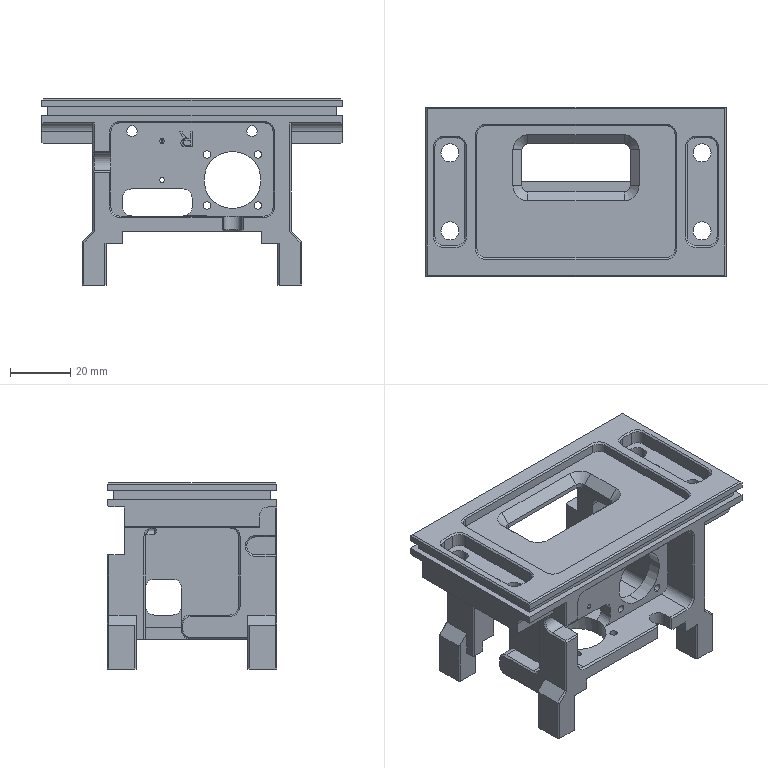NC program | Mastercam | posted with a generic post | part box 100 x 56.5 x 62 mm
Lines 31428 to 33708 of 47040, first 1881 of 2281 lines:
N7300 T16 M6
N7310 G0 G90 G17 G54 X59.62 Y2.263 A0. S5000 M3
N7320 G43 H16 Z20. M8
N7330 Z1.
N7340 G1 Z-28.5 F600.
N7350 X58.489 Y1.131 F1000.
N7360 G3 X58.02 Y0. I1.131 J-1.131
N7370 G1 Y-31.
N7380 G2 X50. Y-39.02 I-8.02 J0.
N7390 G1 X-50.
N7400 G2 X-58.02 Y-31. I0. J8.02
N7410 G1 Y31.
N7420 G2 X-50. Y39.02 I8.02 J0.
N7430 G1 X50.
N7440 G2 X58.02 Y31. I0. J-8.02
N7450 G1 Y0.
N7460 Y-.5
N7470 G3 X58.489 Y-1.631 I1.6 J0.
N7480 G1 X59.62 Y-2.763
N7490 G0 Z20.
N7500 Y2.263
N7510 Z1.
N7520 G1 Z-28.5 F600.
N7530 X58.489 Y1.131 F1000.
N7540 G3 X58.02 Y0. I1.131 J-1.131
N7550 G1 Y-31.
N7560 G2 X50. Y-39.02 I-8.02 J0.
N7570 G1 X-50.
N7580 G2 X-58.02 Y-31. I0. J8.02
N7590 G1 Y31.
N7600 G2 X-50. Y39.02 I8.02 J0.
N7610 G1 X50.
N7620 G2 X58.02 Y31. I0. J-8.02
N7630 G1 Y0.
N7640 Y-.5
N7650 G3 X58.489 Y-1.631 I1.6 J0.
N7660 G1 X59.62 Y-2.763
N7670 Y2.263
N7680 Z-57. F600.
N7690 X58.489 Y1.131 F1000.
N7700 G3 X58.02 Y0. I1.131 J-1.131
N7710 G1 Y-31.
N7720 G2 X50. Y-39.02 I-8.02 J0.
N7730 G1 X-50.
N7740 G2 X-58.02 Y-31. I0. J8.02
N7750 G1 Y31.
N7760 G2 X-50. Y39.02 I8.02 J0.
N7770 G1 X50.
N7780 G2 X58.02 Y31. I0. J-8.02
N7790 G1 Y0.
N7800 Y-.5
N7810 G3 X58.489 Y-1.631 I1.6 J0.
N7820 G1 X59.62 Y-2.763
N7830 G0 Z20.
N7840 Y2.263
N7850 Z-27.5
N7860 G1 Z-57. F600.
N7870 X58.489 Y1.131 F1000.
N7880 G3 X58.02 Y0. I1.131 J-1.131
N7890 G1 Y-31.
N7900 G2 X50. Y-39.02 I-8.02 J0.
N7910 G1 X-50.
N7920 G2 X-58.02 Y-31. I0. J8.02
N7930 G1 Y31.
N7940 G2 X-50. Y39.02 I8.02 J0.
N7950 G1 X50.
N7960 G2 X58.02 Y31. I0. J-8.02
N7970 G1 Y0.
N7980 Y-.5
N7990 G3 X58.489 Y-1.631 I1.6 J0.
N8000 G1 X59.62 Y-2.763
N8010 G0 Z20.
N8020 M5
N8030 G91 G28 Z0. M9
N8040 A0.
N8050 M01
N8060 T5 M6
N8070 G0 G90 G17 G54 X50. Y-31.65 A0. S6500 M3
N8080 G43 H5 Z20. M8
N8090 Z1.
N8100 G1 Z-.75 F600.
N8110 X-50. F1000.
N8120 G2 X-50.65 Y-31. I0. J.65
N8130 G1 Y31.
N8140 G2 X-50. Y31.65 I.65 J0.
N8150 G1 X50.
N8160 G2 X50.65 Y31. I0. J-.65
N8170 G1 Y-31.
N8180 G2 X50. Y-31.65 I-.65 J0.
N8190 G0 Z20.
N8200 Y-26.15
N8210 Z1.
N8220 G1 Z-.75 F600.
N8230 X-50. F1000.
N8240 G0 Z20.
N8250 Y-27.85
N8260 Z1.
N8270 G1 Z-.75 F600.
N8280 X50. F1000.
N8290 G0 Z20.
N8300 X-13.5 Y4.85
N8310 Z1.
N8320 G1 Z-12.75 F600.
N8330 G3 X-22.35 Y-4. I0. J-8.85 F1000.
N8340 X-13.5 Y-12.85 I8.85 J0.
N8350 X-4.65 Y-4. I0. J8.85
N8360 X-13.5 Y4.85 I-8.85 J0.
N8370 G0 Z20.
N8380 X.65 Y5.
N8390 Z1.
N8400 G1 Z-12.75 F600.
N8410 Y2. F1000.
N8420 G3 X3. Y-.35 I2.35 J0.
N8430 G1 X20.2
N8440 G3 X22.55 Y2. I0. J2.35
N8450 G1 Y5.
N8460 G0 Z20.
N8470 X12.166 Y6.95
N8480 Z1.
N8490 G1 Z-1. F600.
N8500 X11.883 Y7.232 F1000.
N8510 G3 X11.6 Y7.35 I-.283 J-.282
N8520 G1 X2.926
N8530 X-24.
N8540 G3 X-26.35 Y5. I0. J-2.35
N8550 G1 Y-20.
N8560 G3 X-24. Y-22.35 I2.35 J0.
N8570 G1 X24.
N8580 G3 X26.35 Y-20. I0. J2.35
N8590 G1 Y5.
N8600 G3 X24. Y7.35 I-2.35 J0.
N8610 G1 X20.274
N8620 X11.6
N8630 X11.1
N8640 G3 X10.817 Y7.232 I0. J-.4
N8650 G1 X10.534 Y6.95
N8660 G0 Z20.
N8670 S6000 M3
N8680 X-22. Y4.5
N8690 G98 G81 Z-12.7 R-11. F200.
N8700 Y-12.5
N8710 X-5. Y4.5
N8720 Y-12.5
N8730 X10. Y-4.
N8740 Y-17.
N8750 X-20. Y-20.3
N8760 X20.
N8770 G80
N8780 M5
N8790 G91 G0 G28 Z0. M9
N8800 A0.
N8810 M01
N8820 T20 M6
N8830 G0 G90 G17 G54 X-104.75 Y23.248 A0. S4000 M3
N8840 G43 H20 Z20. M8
N8850 Z11.
N8860 G1 Z9.34 F600.
N8870 X73.25 F2000.
N8880 G2 X96.498 Y0. I0. J-23.248
N8890 X73.25 Y-23.248 I-23.248 J0.
N8900 G1 X-104.75
N8910 G0 Z20.
N8920 Y23.248
N8930 Z10.34
N8940 G1 Z8.68 F600.
N8950 X73.25 F2000.
N8960 G2 X96.498 Y0. I0. J-23.248
N8970 X73.25 Y-23.248 I-23.248 J0.
N8980 G1 X-104.75
N8990 G0 Z20.
N9000 Y23.248
N9010 Z9.68
N9020 G1 Z8.02 F600.
N9030 X73.25 F2000.
N9040 G2 X96.498 Y0. I0. J-23.248
N9050 X73.25 Y-23.248 I-23.248 J0.
N9060 G1 X-104.75
N9070 G0 Z20.
N9080 Y23.248
N9090 Z9.02
N9100 G1 Z7.36 F600.
N9110 X73.25 F2000.
N9120 G2 X96.498 Y0. I0. J-23.248
N9130 X73.25 Y-23.248 I-23.248 J0.
N9140 G1 X-104.75
N9150 G0 Z20.
N9160 Y23.248
N9170 Z8.36
N9180 G1 Z6.7 F600.
N9190 X73.25 F2000.
N9200 G2 X96.498 Y0. I0. J-23.248
N9210 X73.25 Y-23.248 I-23.248 J0.
N9220 G1 X-104.75
N9230 G0 Z20.
N9240 Y23.248
N9250 Z7.7
N9260 G1 Z6.04 F600.
N9270 X73.25 F2000.
N9280 G2 X96.498 Y0. I0. J-23.248
N9290 X73.25 Y-23.248 I-23.248 J0.
N9300 G1 X-104.75
N9310 G0 Z20.
N9320 Y23.248
N9330 Z7.04
N9340 G1 Z5.38 F600.
N9350 X73.25 F2000.
N9360 G2 X96.498 Y0. I0. J-23.248
N9370 X73.25 Y-23.248 I-23.248 J0.
N9380 G1 X-104.75
N9390 G0 Z20.
N9400 Y23.248
N9410 Z6.38
N9420 G1 Z4.72 F600.
N9430 X73.25 F2000.
N9440 G2 X96.498 Y0. I0. J-23.248
N9450 X73.25 Y-23.248 I-23.248 J0.
N9460 G1 X-104.75
N9470 G0 Z20.
N9480 Y23.248
N9490 Z5.72
N9500 G1 Z4.06 F600.
N9510 X73.25 F2000.
N9520 G2 X96.498 Y0. I0. J-23.248
N9530 X73.25 Y-23.248 I-23.248 J0.
N9540 G1 X-104.75
N9550 G0 Z20.
N9560 Y23.248
N9570 Z5.06
N9580 G1 Z3.4 F600.
N9590 X73.25 F2000.
N9600 G2 X96.498 Y0. I0. J-23.248
N9610 X73.25 Y-23.248 I-23.248 J0.
N9620 G1 X-104.75
N9630 G0 Z20.
N9640 Y23.248
N9650 Z4.4
N9660 G1 Z2.74 F600.
N9670 X73.25 F2000.
N9680 G2 X96.498 Y0. I0. J-23.248
N9690 X73.25 Y-23.248 I-23.248 J0.
N9700 G1 X-104.75
N9710 G0 Z20.
N9720 Y23.248
N9730 Z3.74
N9740 G1 Z2.08 F600.
N9750 X73.25 F2000.
N9760 G2 X96.498 Y0. I0. J-23.248
N9770 X73.25 Y-23.248 I-23.248 J0.
N9780 G1 X-104.75
N9790 G0 Z20.
N9800 Y23.248
N9810 Z3.08
N9820 G1 Z1.42 F600.
N9830 X73.25 F2000.
N9840 G2 X96.498 Y0. I0. J-23.248
N9850 X73.25 Y-23.248 I-23.248 J0.
N9860 G1 X-104.75
N9870 G0 Z20.
N9880 Y23.248
N9890 Z2.42
N9900 G1 Z.76 F600.
N9910 X73.25 F2000.
N9920 G2 X96.498 Y0. I0. J-23.248
N9930 X73.25 Y-23.248 I-23.248 J0.
N9940 G1 X-104.75
N9950 G0 Z20.
N9960 Y23.248
N9970 Z1.76
N9980 G1 Z.1 F600.
N9990 X73.25 F2000.
N100 G2 X96.498 Y0. I0. J-23.248
N110 X73.25 Y-23.248 I-23.248 J0.
N120 G1 X-104.75
N130 G0 Z20.
N140 Y23.248
N150 Z1.1
N160 G1 Z0. F600.
N170 X73.25 F1000.
N180 G2 X96.498 Y0. I0. J-23.248
N190 X73.25 Y-23.248 I-23.248 J0.
N200 G1 X-104.75
N210 G0 Z20.
N220 M5
N230 G91 G28 Z0. M9
N240 A0.
N250 M01
N260 T11 M6
N270 G0 G90 G17 G54 X57. Y-13.1 A0. S8000 M3
N280 G43 H11 Z20. M8
N290 Z1.
N300 G1 Z-.628 F600.
N310 X50. F4000.
N320 X-50.
N330 X-57.
N340 Z-1.256 F600.
N350 X-50. F4000.
N360 X50.
N370 X57.
N380 Z-1.883 F600.
N390 X50. F4000.
N400 X-50.
N410 X-57.
N420 Z-2.511 F600.
N430 X-50. F4000.
N440 X50.
N450 X57.
N460 Z-3.139 F600.
N470 X50. F4000.
N480 X-50.
N490 X-57.
N500 Z-3.767 F600.
N510 X-50. F4000.
N520 X50.
N530 X57.
N540 Z-4.394 F600.
N550 X50. F4000.
N560 X-50.
N570 X-57.
N580 Z-5.022 F600.
N590 X-50. F4000.
N600 X50.
N610 X57.
N620 Z-5.65 F600.
N630 X50. F4000.
N640 X-50.
N650 X-57.
N660 G0 Z20.
N670 Y-16.9
N680 Z1.
N690 G1 Z-.628 F600.
N700 X-50. F4000.
N710 X50.
N720 X57.
N730 Z-1.256 F600.
N740 X50. F4000.
N750 X-50.
N760 X-57.
N770 Z-1.883 F600.
N780 X-50. F4000.
N790 X50.
N800 X57.
N810 Z-2.511 F600.
N820 X50. F4000.
N830 X-50.
N840 X-57.
N850 Z-3.139 F600.
N860 X-50. F4000.
N870 X50.
N880 X57.
N890 Z-3.767 F600.
N900 X50. F4000.
N910 X-50.
N920 X-57.
N930 Z-4.394 F600.
N940 X-50. F4000.
N950 X50.
N960 X57.
N970 Z-5.022 F600.
N980 X50. F4000.
N990 X-50.
N1000 X-57.
N1010 Z-5.65 F600.
N1020 X-50. F4000.
N1030 X50.
N1040 X57.
N1050 G0 Z20.
N1060 M5
N1070 G91 G28 Z0. M9
N1080 A0.
N1090 M01
N1100 T12 M6
N1110 G0 G90 G17 G54 X57. Y-13. A0. S8000 M3
N1120 G43 H12 Z20. M8
N1130 Z-4.75
N1140 G1 Z-5.75 F600.
N1150 X50. F1000.
N1160 X-50.
N1170 X-57.
N1180 G0 Z20.
N1190 Y-17.
N1200 Z-4.75
N1210 G1 Z-5.75 F600.
N1220 X-50. F1000.
N1230 X50.
N1240 X57.
N1250 G0 Z20.
N1260 M5
N1270 G91 G28 Z0. M9
N1280 A0.
N1290 M01
N1300 T11 M6
N1310 G0 G90 G17 G54 X2.228 Y-2.835 A0. S8000 M3
N1320 G43 H11 Z20. M8
N1330 Z1.
N1340 G1 Z.325 F600.
N1350 G3 X7.628 Y2.565 Z.073 I0. J5.4 F4000.
N1360 X2.228 Y7.965 Z-.18 I-5.4 J0.
N1370 X-3.172 Y2.565 Z-.432 I0. J-5.4
N1380 X2.228 Y-2.835 Z-.685 I5.4 J0.
N1390 G1 X3.035
N1400 Y-1.165
N1410 X0.
N1420 X-3.035
N1430 Y-2.835
N1440 X2.228
N1450 G2 X2.953 Y-3.418 I0. J-.743
N1460 G1 X3.73 Y-6.941
N1470 G3 X4.455 Y-7.523 I.725 J.16
N1480 G1 X7.723
N1490 Y3.523
N1500 X0.
N1510 X-7.723
N1520 Y-7.523
N1530 X4.455
N1540 G2 X5.18 Y-8.106 I0. J-.743
N1550 G1 X5.957 Y-11.629
N1560 G3 X6.683 Y-12.212 I.726 J.16
N1570 G1 X12.412
N1580 Y8.212
N1590 X0.
N1600 X-12.412
N1610 Y-12.212
N1620 X6.683
N1630 G2 X7.408 Y-12.794 I0. J-.742
N1640 G1 X8.185 Y-16.317
N1650 G3 X8.91 Y-16.9 I.725 J.16
N1660 G1 X17.099
N1670 X17.1 Y12.656
N1680 X17.087 Y12.887
N1690 X16.959 Y12.898
N1700 X0. Y12.9
N1710 X-16.188
N1720 X-17.087 Y12.887
N1730 X-17.1 Y12.656
N1740 Y-16.898
N1750 X-17.099 Y-16.9
N1760 X8.91
N1770 G0 Z20.
N1780 X2.228 Y-2.835
N1790 Z.315
N1800 G1 Z-.36 F600.
N1810 G3 X7.628 Y2.565 Z-.612 I0. J5.4 F4000.
N1820 X2.228 Y7.965 Z-.865 I-5.4 J0.
N1830 X-3.172 Y2.565 Z-1.117 I0. J-5.4
N1840 X2.228 Y-2.835 Z-1.369 I5.4 J0.
N1850 G1 X3.035
N1860 Y-1.165
N1870 X0.
N1880 X-3.035
N1890 Y-2.835
N1900 X2.228
N1910 G2 X2.953 Y-3.418 I0. J-.743
N1920 G1 X3.73 Y-6.941
N1930 G3 X4.455 Y-7.523 I.725 J.16
N1940 G1 X7.723
N1950 Y3.523
N1960 X0.
N1970 X-7.723
N1980 Y-7.523
N1990 X4.455
N2000 G2 X5.18 Y-8.106 I0. J-.743
N2010 G1 X5.957 Y-11.629
N2020 G3 X6.683 Y-12.212 I.726 J.16
N2030 G1 X12.412
N2040 Y8.212
N2050 X0.
N2060 X-12.412
N2070 Y-12.212
N2080 X6.683
N2090 G2 X7.408 Y-12.794 I0. J-.742
N2100 G1 X8.185 Y-16.317
N2110 G3 X8.91 Y-16.9 I.725 J.16
N2120 G1 X17.099
N2130 X17.1 Y12.656
N2140 X17.087 Y12.887
N2150 X16.959 Y12.898
N2160 X0. Y12.9
N2170 X-16.188
N2180 X-17.087 Y12.887
N2190 X-17.1 Y12.656
N2200 Y-16.898
N2210 X-17.099 Y-16.9
N2220 X8.91
N2230 G0 Z20.
N2240 X2.228 Y-2.835
N2250 Z-.369
N2260 G1 Z-1.044 F600.
N2270 G3 X7.628 Y2.565 Z-1.297 I0. J5.4 F4000.
N2280 X2.228 Y7.965 Z-1.549 I-5.4 J0.
N2290 X-3.172 Y2.565 Z-1.802 I0. J-5.4
N2300 X2.228 Y-2.835 Z-2.054 I5.4 J0.
N2310 G1 X3.035
N2320 Y-1.165
N2330 X0.
N2340 X-3.035
N2350 Y-2.835
N2360 X2.228
N2370 G2 X2.953 Y-3.418 I0. J-.743
N2380 G1 X3.73 Y-6.941
N2390 G3 X4.455 Y-7.523 I.725 J.16
N2400 G1 X7.723
N2410 Y3.523
N2420 X0.
N2430 X-7.723
N2440 Y-7.523
N2450 X4.455
N2460 G2 X5.18 Y-8.106 I0. J-.743
N2470 G1 X5.957 Y-11.629
N2480 G3 X6.683 Y-12.212 I.726 J.16
N2490 G1 X12.412
N2500 Y8.212
N2510 X0.
N2520 X-12.412
N2530 Y-12.212
N2540 X6.683
N2550 G2 X7.408 Y-12.794 I0. J-.742
N2560 G1 X8.185 Y-16.317
N2570 G3 X8.91 Y-16.9 I.725 J.16
N2580 G1 X17.099
N2590 X17.1 Y12.656
N2600 X17.087 Y12.887
N2610 X16.959 Y12.898
N2620 X0. Y12.9
N2630 X-16.188
N2640 X-17.087 Y12.887
N2650 X-17.1 Y12.656
N2660 Y-16.898
N2670 X-17.099 Y-16.9
N2680 X8.91
N2690 G0 Z20.
N2700 X2.228 Y-2.835
N2710 Z-1.054
N2720 G1 Z-1.729 F600.
N2730 G3 X7.628 Y2.565 Z-1.982 I0. J5.4 F4000.
N2740 X2.228 Y7.965 Z-2.234 I-5.4 J0.
N2750 X-3.172 Y2.565 Z-2.486 I0. J-5.4
N2760 X2.228 Y-2.835 Z-2.739 I5.4 J0.
N2770 G1 X3.035
N2780 Y-1.165
N2790 X0.
N2800 X-3.035
N2810 Y-2.835
N2820 X2.228
N2830 G2 X2.953 Y-3.418 I0. J-.743
N2840 G1 X3.73 Y-6.941
N2850 G3 X4.455 Y-7.523 I.725 J.16
N2860 G1 X7.723
N2870 Y3.523
N2880 X0.
N2890 X-7.723
N2900 Y-7.523
N2910 X4.455
N2920 G2 X5.18 Y-8.106 I0. J-.743
N2930 G1 X5.957 Y-11.629
N2940 G3 X6.683 Y-12.212 I.726 J.16
N2950 G1 X12.412
N2960 Y8.212
N2970 X0.
N2980 X-12.412
N2990 Y-12.212
N3000 X6.683
N3010 G2 X7.408 Y-12.794 I0. J-.742
N3020 G1 X8.185 Y-16.317
N3030 G3 X8.91 Y-16.9 I.725 J.16
N3040 G1 X17.099
N3050 X17.1 Y12.656
N3060 X17.087 Y12.887
N3070 X16.959 Y12.898
N3080 X0. Y12.9
N3090 X-16.188
N3100 X-17.087 Y12.887
N3110 X-17.1 Y12.656
N3120 Y-16.898
N3130 X-17.099 Y-16.9
N3140 X8.91
N3150 G0 Z20.
N3160 X2.228 Y-2.835
N3170 Z-1.739
N3180 G1 Z-2.414 F600.
N3190 G3 X7.628 Y2.565 Z-2.666 I0. J5.4 F4000.
N3200 X2.228 Y7.965 Z-2.919 I-5.4 J0.
N3210 X-3.172 Y2.565 Z-3.171 I0. J-5.4
N3220 X2.228 Y-2.835 Z-3.424 I5.4 J0.
N3230 G1 X3.035
N3240 Y-1.165
N3250 X0.
N3260 X-3.035
N3270 Y-2.835
N3280 X2.228
N3290 G2 X2.953 Y-3.418 I0. J-.743
N3300 G1 X3.73 Y-6.941
N3310 G3 X4.455 Y-7.523 I.725 J.16
N3320 G1 X7.723
N3330 Y3.523
N3340 X0.
N3350 X-7.723
N3360 Y-7.523
N3370 X4.455
N3380 G2 X5.18 Y-8.106 I0. J-.743
N3390 G1 X5.957 Y-11.629
N3400 G3 X6.683 Y-12.212 I.726 J.16
N3410 G1 X12.412
N3420 Y8.212
N3430 X0.
N3440 X-12.412
N3450 Y-12.212
N3460 X6.683
N3470 G2 X7.408 Y-12.794 I0. J-.742
N3480 G1 X8.185 Y-16.317
N3490 G3 X8.91 Y-16.9 I.725 J.16
N3500 G1 X17.099
N3510 X17.1 Y12.656
N3520 X17.087 Y12.887
N3530 X16.959 Y12.898
N3540 X0. Y12.9
N3550 X-16.188
N3560 X-17.087 Y12.887
N3570 X-17.1 Y12.656
N3580 Y-16.898
N3590 X-17.099 Y-16.9
N3600 X8.91
N3610 G0 Z20.
N3620 X2.228 Y-2.835
N3630 Z-2.424
N3640 G1 Z-3.099 F600.
N3650 G3 X7.628 Y2.565 Z-3.351 I0. J5.4 F4000.
N3660 X2.228 Y7.965 Z-3.603 I-5.4 J0.
N3670 X-3.172 Y2.565 Z-3.856 I0. J-5.4
N3680 X2.228 Y-2.835 Z-4.108 I5.4 J0.
N3690 G1 X3.035
N3700 Y-1.165
N3710 X0.
N3720 X-3.035
N3730 Y-2.835
N3740 X2.228
N3750 G2 X2.953 Y-3.418 I0. J-.743
N3760 G1 X3.73 Y-6.941
N3770 G3 X4.455 Y-7.523 I.725 J.16
N3780 G1 X7.723
N3790 Y3.523
N3800 X0.
N3810 X-7.723
N3820 Y-7.523
N3830 X4.455
N3840 G2 X5.18 Y-8.106 I0. J-.743
N3850 G1 X5.957 Y-11.629
N3860 G3 X6.683 Y-12.212 I.726 J.16
N3870 G1 X12.412
N3880 Y8.212
N3890 X0.
N3900 X-12.412
N3910 Y-12.212
N3920 X6.683
N3930 G2 X7.408 Y-12.794 I0. J-.742
N3940 G1 X8.185 Y-16.317
N3950 G3 X8.91 Y-16.9 I.725 J.16
N3960 G1 X17.099
N3970 X17.1 Y12.656
N3980 X17.087 Y12.887
N3990 X16.959 Y12.898
N4000 X0. Y12.9
N4010 X-16.188
N4020 X-17.087 Y12.887
N4030 X-17.1 Y12.656
N4040 Y-16.898
N4050 X-17.099 Y-16.9
N4060 X8.91
N4070 G0 Z20.
N4080 X2.228 Y-2.835
N4090 Z-3.108
N4100 G1 Z-3.783 F600.
N4110 G3 X7.628 Y2.565 Z-4.036 I0. J5.4 F4000.
N4120 X2.228 Y7.965 Z-4.288 I-5.4 J0.
N4130 X-3.172 Y2.565 Z-4.541 I0. J-5.4
N4140 X2.228 Y-2.835 Z-4.793 I5.4 J0.
N4150 G1 X3.035
N4160 Y-1.165
N4170 X0.
N4180 X-3.035
N4190 Y-2.835
N4200 X2.228
N4210 G2 X2.953 Y-3.418 I0. J-.743
N4220 G1 X3.73 Y-6.941
N4230 G3 X4.455 Y-7.523 I.725 J.16
N4240 G1 X7.723
N4250 Y3.523
N4260 X0.
N4270 X-7.723
N4280 Y-7.523
N4290 X4.455
N4300 G2 X5.18 Y-8.106 I0. J-.743
N4310 G1 X5.957 Y-11.629
N4320 G3 X6.683 Y-12.212 I.726 J.16
N4330 G1 X12.412
N4340 Y8.212
N4350 X0.
N4360 X-12.412
N4370 Y-12.212
N4380 X6.683
N4390 G2 X7.408 Y-12.794 I0. J-.742
N4400 G1 X8.185 Y-16.317
N4410 G3 X8.91 Y-16.9 I.725 J.16
N4420 G1 X17.099
N4430 X17.1 Y12.656
N4440 X17.087 Y12.887
N4450 X16.959 Y12.898
N4460 X0. Y12.9
N4470 X-16.188
N4480 X-17.087 Y12.887
N4490 X-17.1 Y12.656
N4500 Y-16.898
N4510 X-17.099 Y-16.9
N4520 X8.91
N4530 G0 Z20.
N4540 X2.228 Y-2.835
N4550 Z-3.793
N4560 G1 Z-4.468 F600.
N4570 G3 X7.628 Y2.565 Z-4.72 I0. J5.4 F4000.
N4580 X2.228 Y7.965 Z-4.973 I-5.4 J0.
N4590 X-3.172 Y2.565 Z-5.225 I0. J-5.4
N4600 X2.228 Y-2.835 Z-5.478 I5.4 J0.
N4610 G1 X3.035
N4620 Y-1.165
N4630 X0.
N4640 X-3.035
N4650 Y-2.835
N4660 X2.228
N4670 G2 X2.953 Y-3.418 I0. J-.743
N4680 G1 X3.73 Y-6.941
N4690 G3 X4.455 Y-7.523 I.725 J.16
N4700 G1 X7.723
N4710 Y3.523
N4720 X0.
N4730 X-7.723
N4740 Y-7.523
N4750 X4.455
N4760 G2 X5.18 Y-8.106 I0. J-.743
N4770 G1 X5.957 Y-11.629
N4780 G3 X6.683 Y-12.212 I.726 J.16
N4790 G1 X12.412
N4800 Y8.212
N4810 X0.
N4820 X-12.412
N4830 Y-12.212
N4840 X6.683
N4850 G2 X7.408 Y-12.794 I0. J-.742
N4860 G1 X8.185 Y-16.317
N4870 G3 X8.91 Y-16.9 I.725 J.16
N4880 G1 X17.099
N4890 X17.1 Y12.656
N4900 X17.087 Y12.887
N4910 X16.959 Y12.898
N4920 X0. Y12.9
N4930 X-16.188
N4940 X-17.087 Y12.887
N4950 X-17.1 Y12.656
N4960 Y-16.898
N4970 X-17.099 Y-16.9
N4980 X8.91
N4990 G0 Z20.
N5000 X2.228 Y-2.835
N5010 Z-4.478
N5020 G1 Z-5.153 F600.
N5030 G3 X7.628 Y2.565 Z-5.405 I0. J5.4 F4000.
N5040 X2.228 Y7.965 Z-5.658 I-5.4 J0.
N5050 X-3.172 Y2.565 Z-5.91 I0. J-5.4
N5060 X2.228 Y-2.835 Z-6.162 I5.4 J0.
N5070 G1 X3.035
N5080 Y-1.165
N5090 X0.
N5100 X-3.035
N5110 Y-2.835
N5120 X2.228
N5130 G2 X2.953 Y-3.418 I0. J-.743
N5140 G1 X3.73 Y-6.941
N5150 G3 X4.455 Y-7.523 I.725 J.16
N5160 G1 X7.723
N5170 Y3.523
N5180 X0.
N5190 X-7.723
N5200 Y-7.523
N5210 X4.455
N5220 G2 X5.18 Y-8.106 I0. J-.743
N5230 G1 X5.957 Y-11.629
N5240 G3 X6.683 Y-12.212 I.726 J.16
N5250 G1 X12.412
N5260 Y8.212
N5270 X0.
N5280 X-12.412
N5290 Y-12.212
N5300 X6.683
N5310 G2 X7.408 Y-12.794 I0. J-.742
N5320 G1 X8.185 Y-16.317
N5330 G3 X8.91 Y-16.9 I.725 J.16
N5340 G1 X17.099
N5350 X17.1 Y12.656
N5360 X17.087 Y12.887
N5370 X16.959 Y12.898
N5380 X0. Y12.9
N5390 X-16.188
N5400 X-17.087 Y12.887
N5410 X-17.1 Y12.656
N5420 Y-16.898
N5430 X-17.099 Y-16.9
N5440 X8.91
N5450 G0 Z20.
N5460 X2.228 Y-2.835
N5470 Z-5.162
N5480 G1 Z-5.838 F600.
N5490 G3 X7.628 Y2.565 Z-6.09 I0. J5.4 F4000.
N5500 X2.228 Y7.965 Z-6.342 I-5.4 J0.
N5510 X-3.172 Y2.565 Z-6.595 I0. J-5.4
N5520 X2.228 Y-2.835 Z-6.847 I5.4 J0.
N5530 G1 X3.035
N5540 Y-1.165
N5550 X0.
N5560 X-3.035
N5570 Y-2.835
N5580 X2.228
N5590 G2 X2.953 Y-3.418 I0. J-.743
N5600 G1 X3.73 Y-6.941
N5610 G3 X4.455 Y-7.523 I.725 J.16
N5620 G1 X7.723
N5630 Y3.523
N5640 X0.
N5650 X-7.723
N5660 Y-7.523
N5670 X4.455
N5680 G2 X5.18 Y-8.106 I0. J-.743
N5690 G1 X5.957 Y-11.629
N5700 G3 X6.683 Y-12.212 I.726 J.16
N5710 G1 X12.412
N5720 Y8.212
N5730 X0.
N5740 X-12.412
N5750 Y-12.212
N5760 X6.683
N5770 G2 X7.408 Y-12.794 I0. J-.742
N5780 G1 X8.185 Y-16.317
N5790 G3 X8.91 Y-16.9 I.725 J.16
N5800 G1 X17.099
N5810 X17.1 Y12.656
N5820 X17.087 Y12.887
N5830 X16.959 Y12.898
N5840 X0. Y12.9
N5850 X-16.188
N5860 X-17.087 Y12.887
N5870 X-17.1 Y12.656
N5880 Y-16.898
N5890 X-17.099 Y-16.9
N5900 X8.91
N5910 G0 Z20.
N5920 X2.228 Y-2.835
N5930 Z-5.847
N5940 G1 Z-6.522 F600.
N5950 G3 X7.628 Y2.565 Z-6.775 I0. J5.4 F4000.
N5960 X2.228 Y7.965 Z-7.027 I-5.4 J0.
N5970 X-3.172 Y2.565 Z-7.28 I0. J-5.4
N5980 X2.228 Y-2.835 Z-7.532 I5.4 J0.
N5990 G1 X3.035
N6000 Y-1.165
N6010 X0.
N6020 X-3.035
N6030 Y-2.835
N6040 X2.228
N6050 G2 X2.953 Y-3.418 I0. J-.743
N6060 G1 X3.73 Y-6.941
N6070 G3 X4.455 Y-7.523 I.725 J.16
N6080 G1 X7.723
N6090 Y3.523
N6100 X0.
N6110 X-7.723
N6120 Y-7.523
N6130 X4.455
N6140 G2 X5.18 Y-8.106 I0. J-.743
N6150 G1 X5.957 Y-11.629
N6160 G3 X6.683 Y-12.212 I.726 J.16
N6170 G1 X12.412
N6180 Y8.212
N6190 X0.
N6200 X-12.412
N6210 Y-12.212
N6220 X6.683
N6230 G2 X7.408 Y-12.794 I0. J-.742
N6240 G1 X8.185 Y-16.317
N6250 G3 X8.91 Y-16.9 I.725 J.16
N6260 G1 X17.099
N6270 X17.1 Y12.656
N6280 X17.087 Y12.887
N6290 X16.959 Y12.898
N6300 X0. Y12.9
N6310 X-16.188
N6320 X-17.087 Y12.887
N6330 X-17.1 Y12.656
N6340 Y-16.898
N6350 X-17.099 Y-16.9
N6360 X8.91
N6370 G0 Z20.
N6380 X2.228 Y-2.835
N6390 Z-6.532
N6400 G1 Z-7.207 F600.
N6410 G3 X7.628 Y2.565 Z-7.459 I0. J5.4 F4000.
N6420 X2.228 Y7.965 Z-7.712 I-5.4 J0.
N6430 X-3.172 Y2.565 Z-7.964 I0. J-5.4
N6440 X2.228 Y-2.835 Z-8.217 I5.4 J0.
N6450 G1 X3.035
N6460 Y-1.165
N6470 X0.
N6480 X-3.035
N6490 Y-2.835
N6500 X2.228
N6510 G2 X2.953 Y-3.418 I0. J-.743
N6520 G1 X3.73 Y-6.941
N6530 G3 X4.455 Y-7.523 I.725 J.16
N6540 G1 X7.723
N6550 Y3.523
N6560 X0.
N6570 X-7.723
N6580 Y-7.523
N6590 X4.455
N6600 G2 X5.18 Y-8.106 I0. J-.743
N6610 G1 X5.957 Y-11.629
N6620 G3 X6.683 Y-12.212 I.726 J.16
N6630 G1 X12.412
N6640 Y8.212
N6650 X0.
N6660 X-12.412
N6670 Y-12.212
N6680 X6.683
N6690 G2 X7.408 Y-12.794 I0. J-.742
N6700 G1 X8.185 Y-16.317
N6710 G3 X8.91 Y-16.9 I.725 J.16
N6720 G1 X17.099
N6730 X17.1 Y12.656
N6740 X17.087 Y12.887
N6750 X16.959 Y12.898
N6760 X0. Y12.9
N6770 X-16.188
N6780 X-17.087 Y12.887
N6790 X-17.1 Y12.656
N6800 Y-16.898
N6810 X-17.099 Y-16.9
N6820 X8.91
N6830 G0 Z20.
N6840 X2.228 Y-2.835
N6850 Z-7.217
N6860 G1 Z-7.892 F600.
N6870 G3 X7.628 Y2.565 Z-8.144 I0. J5.4 F4000.
N6880 X2.228 Y7.965 Z-8.397 I-5.4 J0.
N6890 X-3.172 Y2.565 Z-8.649 I0. J-5.4
N6900 X2.228 Y-2.835 Z-8.901 I5.4 J0.
N6910 G1 X3.035
N6920 Y-1.165
N6930 X0.
N6940 X-3.035
N6950 Y-2.835
N6960 X2.228
N6970 G2 X2.953 Y-3.418 I0. J-.743
N6980 G1 X3.73 Y-6.941
N6990 G3 X4.455 Y-7.523 I.725 J.16
N7000 G1 X7.723
N7010 Y3.523
N7020 X0.
N7030 X-7.723
N7040 Y-7.523
N7050 X4.455
N7060 G2 X5.18 Y-8.106 I0. J-.743
N7070 G1 X5.957 Y-11.629
N7080 G3 X6.683 Y-12.212 I.726 J.16
N7090 G1 X12.412
N7100 Y8.212
N7110 X0.
N7120 X-12.412
N7130 Y-12.212
N7140 X6.683
N7150 G2 X7.408 Y-12.794 I0. J-.742
N7160 G1 X8.185 Y-16.317
N7170 G3 X8.91 Y-16.9 I.725 J.16
N7180 G1 X17.099
N7190 X17.1 Y12.656
N7200 X17.087 Y12.887
N7210 X16.959 Y12.898
N7220 X0. Y12.9
N7230 X-16.188
N7240 X-17.087 Y12.887
N7250 X-17.1 Y12.656
N7260 Y-16.898
N7270 X-17.099 Y-16.9
N7280 X8.91
N7290 G0 Z20.
N7300 X2.228 Y-2.835
N7310 Z-7.901
N7320 G1 Z-8.576 F600.
N7330 G3 X7.628 Y2.565 Z-8.829 I0. J5.4 F4000.
N7340 X2.228 Y7.965 Z-9.081 I-5.4 J0.
N7350 X-3.172 Y2.565 Z-9.334 I0. J-5.4
N7360 X2.228 Y-2.835 Z-9.586 I5.4 J0.
N7370 G1 X3.035
N7380 Y-1.165
N7390 X0.
N7400 X-3.035
N7410 Y-2.835
N7420 X2.228
N7430 G2 X2.953 Y-3.418 I0. J-.743
N7440 G1 X3.73 Y-6.941
N7450 G3 X4.455 Y-7.523 I.725 J.16
N7460 G1 X7.723
N7470 Y3.523
N7480 X0.
N7490 X-7.723
N7500 Y-7.523
N7510 X4.455
N7520 G2 X5.18 Y-8.106 I0. J-.743
N7530 G1 X5.957 Y-11.629
N7540 G3 X6.683 Y-12.212 I.726 J.16
N7550 G1 X12.412
N7560 Y8.212
N7570 X0.
N7580 X-12.412
N7590 Y-12.212
N7600 X6.683
N7610 G2 X7.408 Y-12.794 I0. J-.742
N7620 G1 X8.185 Y-16.317
N7630 G3 X8.91 Y-16.9 I.725 J.16
N7640 G1 X17.099
N7650 X17.1 Y12.656
N7660 X17.087 Y12.887
N7670 X16.959 Y12.898
N7680 X0. Y12.9
N7690 X-16.188
N7700 X-17.087 Y12.887
N7710 X-17.1 Y12.656
N7720 Y-16.898
N7730 X-17.099 Y-16.9
N7740 X8.91
N7750 G0 Z20.
N7760 X2.228 Y-2.835
N7770 Z-8.586
N7780 G1 Z-9.261 F600.
N7790 G3 X7.628 Y2.565 Z-9.514 I0. J5.4 F4000.
N7800 X2.228 Y7.965 Z-9.766 I-5.4 J0.
N7810 X-3.172 Y2.565 Z-10.018 I0. J-5.4
N7820 X2.228 Y-2.835 Z-10.271 I5.4 J0.
N7830 G1 X3.035
N7840 Y-1.165
N7850 X0.
N7860 X-3.035
N7870 Y-2.835
N7880 X2.228
N7890 G2 X2.953 Y-3.418 I0. J-.743
N7900 G1 X3.73 Y-6.941
N7910 G3 X4.455 Y-7.523 I.725 J.16
N7920 G1 X7.723
N7930 Y3.523
N7940 X0.
N7950 X-7.723
N7960 Y-7.523
N7970 X4.455
N7980 G2 X5.18 Y-8.106 I0. J-.743
N7990 G1 X5.957 Y-11.629
N8000 G3 X6.683 Y-12.212 I.726 J.16
N8010 G1 X12.412
N8020 Y8.212
N8030 X0.
N8040 X-12.412
N8050 Y-12.212
N8060 X6.683
N8070 G2 X7.408 Y-12.794 I0. J-.742
N8080 G1 X8.185 Y-16.317
N8090 G3 X8.91 Y-16.9 I.725 J.16
N8100 G1 X17.099
N8110 X17.1 Y12.656
N8120 X17.087 Y12.887
N8130 X16.959 Y12.898
N8140 X0. Y12.9
N8150 X-16.188
N8160 X-17.087 Y12.887
N8170 X-17.1 Y12.656
N8180 Y-16.898
N8190 X-17.099 Y-16.9
N8200 X8.91
N8210 G0 Z20.
N8220 X2.228 Y-2.835
N8230 Z-9.271
N8240 G1 Z-9.946 F600.
N8250 G3 X7.628 Y2.565 Z-10.198 I0. J5.4 F4000.
N8260 X2.228 Y7.965 Z-10.451 I-5.4 J0.
N8270 X-3.172 Y2.565 Z-10.703 I0. J-5.4
N8280 X2.228 Y-2.835 Z-10.956 I5.4 J0.
N8290 G1 X3.035
N8300 Y-1.165
N8310 X0.
N8320 X-3.035
N8330 Y-2.835
N8340 X2.228
N8350 G2 X2.953 Y-3.418 I0. J-.743
N8360 G1 X3.73 Y-6.941
N8370 G3 X4.455 Y-7.523 I.725 J.16
N8380 G1 X7.723
N8390 Y3.523
N8400 X0.
N8410 X-7.723
N8420 Y-7.523
N8430 X4.455
N8440 G2 X5.18 Y-8.106 I0. J-.743
N8450 G1 X5.957 Y-11.629
N8460 G3 X6.683 Y-12.212 I.726 J.16
N8470 G1 X12.412
N8480 Y8.212
N8490 X0.
N8500 X-12.412
N8510 Y-12.212
N8520 X6.683
N8530 G2 X7.408 Y-12.794 I0. J-.742
N8540 G1 X8.185 Y-16.317
N8550 G3 X8.91 Y-16.9 I.725 J.16
N8560 G1 X17.099
N8570 X17.1 Y12.656
N8580 X17.087 Y12.887
N8590 X16.959 Y12.898
N8600 X0. Y12.9
N8610 X-16.188
N8620 X-17.087 Y12.887
N8630 X-17.1 Y12.656
N8640 Y-16.898
N8650 X-17.099 Y-16.9
N8660 X8.91
N8670 G0 Z20.
N8680 X2.228 Y-2.835
N8690 Z-9.956
N8700 G1 Z-10.631 F600.
N8710 G3 X7.628 Y2.565 Z-10.883 I0. J5.4 F4000.
N8720 X2.228 Y7.965 Z-11.135 I-5.4 J0.
N8730 X-3.172 Y2.565 Z-11.388 I0. J-5.4
N8740 X2.228 Y-2.835 Z-11.64 I5.4 J0.
N8750 G1 X3.035
N8760 Y-1.165
N8770 X0.
N8780 X-3.035
N8790 Y-2.835
N8800 X2.228
N8810 G2 X2.953 Y-3.418 I0. J-.743
N8820 G1 X3.73 Y-6.941
N8830 G3 X4.455 Y-7.523 I.725 J.16
N8840 G1 X7.723
N8850 Y3.523
N8860 X0.
N8870 X-7.723
N8880 Y-7.523
N8890 X4.455
N8900 G2 X5.18 Y-8.106 I0. J-.743
N8910 G1 X5.957 Y-11.629
N8920 G3 X6.683 Y-12.212 I.726 J.16
N8930 G1 X12.412
N8940 Y8.212
N8950 X0.
N8960 X-12.412
N8970 Y-12.212
N8980 X6.683
N8990 G2 X7.408 Y-12.794 I0. J-.742
N9000 G1 X8.185 Y-16.317
N9010 G3 X8.91 Y-16.9 I.725 J.16
N9020 G1 X17.099
N9030 X17.1 Y12.656
N9040 X17.087 Y12.887
N9050 X16.959 Y12.898
N9060 X0. Y12.9
N9070 X-16.188
N9080 X-17.087 Y12.887
N9090 X-17.1 Y12.656
N9100 Y-16.898
N9110 X-17.099 Y-16.9
N9120 X8.91
N9130 G0 Z20.
N9140 X2.228 Y-2.835
N9150 Z-10.64
N9160 G1 Z-11.315 F600.
N9170 G3 X7.628 Y2.565 Z-11.568 I0. J5.4 F4000.
N9180 X2.228 Y7.965 Z-11.82 I-5.4 J0.
N9190 X-3.172 Y2.565 Z-12.073 I0. J-5.4
N9200 X2.228 Y-2.835 Z-12.325 I5.4 J0.
N9210 G1 X3.035
N9220 Y-1.165
N9230 X0.
N9240 X-3.035
N9250 Y-2.835
N9260 X2.228
N9270 G2 X2.953 Y-3.418 I0. J-.743
N9280 G1 X3.73 Y-6.941
N9290 G3 X4.455 Y-7.523 I.725 J.16
N9300 G1 X7.723
N9310 Y3.523
N9320 X0.
N9330 X-7.723
N9340 Y-7.523
N9350 X4.455
N9360 G2 X5.18 Y-8.106 I0. J-.743
N9370 G1 X5.957 Y-11.629
N9380 G3 X6.683 Y-12.212 I.726 J.16
N9390 G1 X12.412
N9400 Y8.212
N9410 X0.
N9420 X-12.412
N9430 Y-12.212
N9440 X6.683
N9450 G2 X7.408 Y-12.794 I0. J-.742
N9460 G1 X8.185 Y-16.317
N9470 G3 X8.91 Y-16.9 I.725 J.16
N9480 G1 X17.099
N9490 X17.1 Y12.656
N9500 X17.087 Y12.887
N9510 X16.959 Y12.898
N9520 X0. Y12.9
N9530 X-16.188
N9540 X-17.087 Y12.887
N9550 X-17.1 Y12.656
N9560 Y-16.898
N9570 X-17.099 Y-16.9
N9580 X8.91
N9590 G0 Z20.
N9600 X2.228 Y-2.835
N9610 Z-11.325
N9620 G1 Z-12. F600.
N9630 G3 X7.628 Y2.565 Z-12.252 I0. J5.4 F4000.
N9640 X2.228 Y7.965 Z-12.505 I-5.4 J0.
N9650 X-3.172 Y2.565 Z-12.757 I0. J-5.4
N9660 X2.228 Y-2.835 Z-13.01 I5.4 J0.
N9670 G1 X3.035
N9680 Y-1.165
N9690 X0.
N9700 X-3.035
N9710 Y-2.835
N9720 X2.228
N9730 G2 X2.953 Y-3.418 I0. J-.743
N9740 G1 X3.73 Y-6.941
N9750 G3 X4.455 Y-7.523 I.725 J.16
N9760 G1 X7.723
N9770 Y3.523
N9780 X0.
N9790 X-7.723
N9800 Y-7.523
N9810 X4.455
N9820 G2 X5.18 Y-8.106 I0. J-.743
N9830 G1 X5.957 Y-11.629
N9840 G3 X6.683 Y-12.212 I.726 J.16
N9850 G1 X12.412
N9860 Y8.212
N9870 X0.
N9880 X-12.412
N9890 Y-12.212
N9900 X6.683
N9910 G2 X7.408 Y-12.794 I0. J-.742
N9920 G1 X8.185 Y-16.317
N9930 G3 X8.91 Y-16.9 I.725 J.16
N9940 G1 X17.099
N9950 X17.1 Y12.656
N9960 X17.087 Y12.887
N9970 X16.959 Y12.898
N9980 X0. Y12.9
N9990 X-16.188
N100 X-17.087 Y12.887
N110 X-17.1 Y12.656
N120 Y-16.898
N130 X-17.099 Y-16.9
N140 X8.91
N150 G0 Z20.
N160 X2.228 Y-2.835
N170 Z-12.01
N180 G1 Z-12.685 F600.
N190 G3 X7.628 Y2.565 Z-12.937 I0. J5.4 F4000.
N200 X2.228 Y7.965 Z-13.19 I-5.4 J0.
N210 X-3.172 Y2.565 Z-13.442 I0. J-5.4
N220 X2.228 Y-2.835 Z-13.694 I5.4 J0.
N230 G1 X3.035
N240 Y-1.165
N250 X0.
N260 X-3.035
N270 Y-2.835
N280 X2.228
N290 G2 X2.953 Y-3.418 I0. J-.743
N300 G1 X3.73 Y-6.941
N310 G3 X4.455 Y-7.523 I.725 J.16
N320 G1 X7.723
N330 Y3.523
N340 X0.
N350 X-7.723
N360 Y-7.523
N370 X4.455
N380 G2 X5.18 Y-8.106 I0. J-.743
N390 G1 X5.957 Y-11.629
N400 G3 X6.683 Y-12.212 I.726 J.16
N410 G1 X12.412
N420 Y8.212
N430 X0.
N440 X-12.412
N450 Y-12.212
N460 X6.683
N470 G2 X7.408 Y-12.794 I0. J-.742
N480 G1 X8.185 Y-16.317
N490 G3 X8.91 Y-16.9 I.725 J.16
N500 G1 X17.099
N510 X17.1 Y12.656
N520 X17.087 Y12.887
N530 X16.959 Y12.898
N540 X0. Y12.9
N550 X-16.188
N560 X-17.087 Y12.887
N570 X-17.1 Y12.656
N580 Y-16.898
N590 X-17.099 Y-16.9
N600 X8.91
N610 G0 Z20.
N620 X2.228 Y-2.835
N630 Z-12.694
N640 G1 Z-13.369 F600.
N650 G3 X7.628 Y2.565 Z-13.622 I0. J5.4 F4000.
N660 X2.228 Y7.965 Z-13.874 I-5.4 J0.
N670 X-3.172 Y2.565 Z-14.127 I0. J-5.4
N680 X2.228 Y-2.835 Z-14.379 I5.4 J0.
N690 G1 X3.035
N700 Y-1.165
N710 X0.
N720 X-3.035
N730 Y-2.835
N740 X2.228
N750 G2 X2.953 Y-3.418 I0. J-.743
N760 G1 X3.73 Y-6.941
N770 G3 X4.455 Y-7.523 I.725 J.16
N780 G1 X7.723
N790 Y3.523
N800 X0.
N810 X-7.723
N820 Y-7.523
N830 X4.455
N840 G2 X5.18 Y-8.106 I0. J-.743
N850 G1 X5.957 Y-11.629
N860 G3 X6.683 Y-12.212 I.726 J.16
N870 G1 X12.412
N880 Y8.212
N890 X0.
N900 X-12.412
N910 Y-12.212
N920 X6.683
N930 G2 X7.408 Y-12.794 I0. J-.742
N940 G1 X8.185 Y-16.317
N950 G3 X8.91 Y-16.9 I.725 J.16
N960 G1 X17.099
N970 X17.1 Y12.656
N980 X17.087 Y12.887
N990 X16.959 Y12.898
N1000 X0. Y12.9
N1010 X-16.188
N1020 X-17.087 Y12.887
N1030 X-17.1 Y12.656
N1040 Y-16.898
N1050 X-17.099 Y-16.9
N1060 X8.91
N1070 G0 Z20.
N1080 X2.228 Y-2.835
N1090 Z-13.379
N1100 G1 Z-14.054 F600.
N1110 G3 X7.628 Y2.565 Z-14.307 I0. J5.4 F4000.
N1120 X2.228 Y7.965 Z-14.559 I-5.4 J0.
N1130 X-3.172 Y2.565 Z-14.811 I0. J-5.4
N1140 X2.228 Y-2.835 Z-15.064 I5.4 J0.
N1150 G1 X3.035
N1160 Y-1.165
N1170 X0.
N1180 X-3.035
N1190 Y-2.835
N1200 X2.228
N1210 G2 X2.953 Y-3.418 I0. J-.743
N1220 G1 X3.73 Y-6.941
N1230 G3 X4.455 Y-7.523 I.725 J.16
N1240 G1 X7.723
N1250 Y3.523
N1260 X0.
N1270 X-7.723
N1280 Y-7.523
N1290 X4.455
N1300 G2 X5.18 Y-8.106 I0. J-.743
N1310 G1 X5.957 Y-11.629
N1320 G3 X6.683 Y-12.212 I.726 J.16
N1330 G1 X12.412
N1340 Y8.212
N1350 X0.
N1360 X-12.412
N1370 Y-12.212
N1380 X6.683
N1390 G2 X7.408 Y-12.794 I0. J-.742
N1400 G1 X8.185 Y-16.317
N1410 G3 X8.91 Y-16.9 I.725 J.16
N1420 G1 X17.099
N1430 X17.1 Y12.656
N1440 X17.087 Y12.887
N1450 X16.959 Y12.898
N1460 X0. Y12.9
N1470 X-16.188
N1480 X-17.087 Y12.887
N1490 X-17.1 Y12.656
N1500 Y-16.898
N1510 X-17.099 Y-16.9
N1520 X8.91
N1530 G0 Z20.
N1540 X2.228 Y-2.835
N1550 Z-14.064
N1560 G1 Z-14.739 F600.
N1570 G3 X7.628 Y2.565 Z-14.991 I0. J5.4 F4000.
N1580 X2.228 Y7.965 Z-15.244 I-5.4 J0.
N1590 X-3.172 Y2.565 Z-15.496 I0. J-5.4
N1600 X2.228 Y-2.835 Z-15.749 I5.4 J0.
N1610 G1 X3.035
N1620 Y-1.165
N1630 X0.
N1640 X-3.035
N1650 Y-2.835
N1660 X2.228
N1670 G2 X2.953 Y-3.418 I0. J-.743
N1680 G1 X3.73 Y-6.941
N1690 G3 X4.455 Y-7.523 I.725 J.16
N1700 G1 X7.723
N1710 Y3.523
N1720 X0.
N1730 X-7.723
N1740 Y-7.523
N1750 X4.455
N1760 G2 X5.18 Y-8.106 I0. J-.743
N1770 G1 X5.957 Y-11.629
N1780 G3 X6.683 Y-12.212 I.726 J.16
N1790 G1 X12.412
N1800 Y8.212
N1810 X0.
N1820 X-12.412
N1830 Y-12.212
N1840 X6.683
N1850 G2 X7.408 Y-12.794 I0. J-.742
N1860 G1 X8.185 Y-16.317
N1870 G3 X8.91 Y-16.9 I.725 J.16
N1880 G1 X17.099
N1890 X17.1 Y12.656
N1900 X17.087 Y12.887
N1910 X16.959 Y12.898
N1920 X0. Y12.9
N1930 X-16.188
N1940 X-17.087 Y12.887
N1950 X-17.1 Y12.656
N1960 Y-16.898
N1970 X-17.099 Y-16.9
N1980 X8.91
N1990 G0 Z20.
N2000 X2.228 Y-2.835
N2010 Z-14.749
N2020 G1 Z-15.424 F600.
N2030 G3 X7.628 Y2.565 Z-15.676 I0. J5.4 F4000.
N2040 X2.228 Y7.965 Z-15.928 I-5.4 J0.
N2050 X-3.172 Y2.565 Z-16.181 I0. J-5.4
N2060 X2.228 Y-2.835 Z-16.433 I5.4 J0.
N2070 G1 X3.035
N2080 Y-1.165
N2090 X0.
N2100 X-3.035
N2110 Y-2.835
N2120 X2.228
N2130 G2 X2.953 Y-3.418 I0. J-.743
N2140 G1 X3.73 Y-6.941
N2150 G3 X4.455 Y-7.523 I.725 J.16
N2160 G1 X7.723
N2170 Y3.523
N2180 X0.
N2190 X-7.723
N2200 Y-7.523
N2210 X4.455
N2220 G2 X5.18 Y-8.106 I0. J-.743
N2230 G1 X5.957 Y-11.629
N2240 G3 X6.683 Y-12.212 I.726 J.16
N2250 G1 X12.412
N2260 Y8.212
N2270 X0.
N2280 X-12.412
N2290 Y-12.212
N2300 X6.683
N2310 G2 X7.408 Y-12.794 I0. J-.742
N2320 G1 X8.185 Y-16.317
N2330 G3 X8.91 Y-16.9 I.725 J.16
N2340 G1 X17.099
N2350 X17.1 Y12.656
N2360 X17.087 Y12.887
N2370 X16.959 Y12.898
N2380 X0. Y12.9
N2390 X-16.188
N2400 X-17.087 Y12.887
N2410 X-17.1 Y12.656
N2420 Y-16.898
N2430 X-17.099 Y-16.9
N2440 X8.91
N2450 G0 Z20.
N2460 X2.228 Y-2.835
N2470 Z-15.433
N2480 G1 Z-16.108 F600.
N2490 G3 X7.628 Y2.565 Z-16.361 I0. J5.4 F4000.
N2500 X2.228 Y7.965 Z-16.613 I-5.4 J0.
N2510 X-3.172 Y2.565 Z-16.866 I0. J-5.4
N2520 X2.228 Y-2.835 Z-17.118 I5.4 J0.
N2530 G1 X3.035
N2540 Y-1.165
N2550 X0.
N2560 X-3.035
N2570 Y-2.835
N2580 X2.228
N2590 G2 X2.953 Y-3.418 I0. J-.743
N2600 G1 X3.73 Y-6.941
N2610 G3 X4.455 Y-7.523 I.725 J.16
N2620 G1 X7.723
N2630 Y3.523
N2640 X0.
N2650 X-7.723
N2660 Y-7.523
N2670 X4.455
N2680 G2 X5.18 Y-8.106 I0. J-.743
N2690 G1 X5.957 Y-11.629
N2700 G3 X6.683 Y-12.212 I.726 J.16
N2710 G1 X12.412
N2720 Y8.212
N2730 X0.
N2740 X-12.412
N2750 Y-12.212
N2760 X6.683
N2770 G2 X7.408 Y-12.794 I0. J-.742
N2780 G1 X8.185 Y-16.317
N2790 G3 X8.91 Y-16.9 I.725 J.16
N2800 G1 X17.099
N2810 X17.1 Y12.656
N2820 X17.087 Y12.887
N2830 X16.959 Y12.898
N2840 X0. Y12.9
N2850 X-16.188
N2860 X-17.087 Y12.887
N2870 X-17.1 Y12.656
N2880 Y-16.898
N2890 X-17.099 Y-16.9
N2900 X8.91
N2910 G0 Z20.
N2920 X2.228 Y-2.835
N2930 Z-16.118
N2940 G1 Z-16.793 F600.
N2950 G3 X7.628 Y2.565 Z-17.045 I0. J5.4 F4000.
N2960 X2.228 Y7.965 Z-17.298 I-5.4 J0.
N2970 X-3.172 Y2.565 Z-17.55 I0. J-5.4
N2980 X2.228 Y-2.835 Z-17.803 I5.4 J0.
N2990 G1 X3.035
N3000 Y-1.165
N3010 X0.
N3020 X-3.035
N3030 Y-2.835
N3040 X2.228
N3050 G2 X2.953 Y-3.418 I0. J-.743
N3060 G1 X3.73 Y-6.941
N3070 G3 X4.455 Y-7.523 I.725 J.16
N3080 G1 X7.723
N3090 Y3.523
N3100 X0.
N3110 X-7.723
N3120 Y-7.523
N3130 X4.455
N3140 G2 X5.18 Y-8.106 I0. J-.743
N3150 G1 X5.957 Y-11.629
N3160 G3 X6.683 Y-12.212 I.726 J.16
N3170 G1 X12.412
N3180 Y8.212
N3190 X0.
N3200 X-12.412
N3210 Y-12.212
N3220 X6.683
N3230 G2 X7.408 Y-12.794 I0. J-.742
N3240 G1 X8.185 Y-16.317
N3250 G3 X8.91 Y-16.9 I.725 J.16
N3260 G1 X17.099
N3270 X17.1 Y12.656
N3280 X17.087 Y12.887
N3290 X16.959 Y12.898
N3300 X0. Y12.9
N3310 X-16.188
N3320 X-17.087 Y12.887
N3330 X-17.1 Y12.656
N3340 Y-16.898
N3350 X-17.099 Y-16.9
N3360 X8.91
N3370 G0 Z20.
N3380 X2.228 Y-2.835
N3390 Z-16.803
N3400 G1 Z-17.478 F600.
N3410 G3 X7.628 Y2.565 Z-17.73 I0. J5.4 F4000.
N3420 X2.228 Y7.965 Z-17.983 I-5.4 J0.
N3430 X-3.172 Y2.565 Z-18.235 I0. J-5.4
N3440 X2.228 Y-2.835 Z-18.488 I5.4 J0.
N3450 G1 X3.035
N3460 Y-1.165
N3470 X0.
N3480 X-3.035
N3490 Y-2.835
N3500 X2.228
N3510 G2 X2.953 Y-3.418 I0. J-.743
N3520 G1 X3.73 Y-6.941
N3530 G3 X4.455 Y-7.523 I.725 J.16
N3540 G1 X7.723
N3550 Y3.523
N3560 X0.
N3570 X-7.723
N3580 Y-7.523
N3590 X4.455
N3600 G2 X5.18 Y-8.106 I0. J-.743
N3610 G1 X5.957 Y-11.629
N3620 G3 X6.683 Y-12.212 I.726 J.16
N3630 G1 X12.412
N3640 Y8.212
N3650 X0.
N3660 X-12.412
N3670 Y-12.212
N3680 X6.683
N3690 G2 X7.408 Y-12.794 I0. J-.742
N3700 G1 X8.185 Y-16.317
N3710 G3 X8.91 Y-16.9 I.725 J.16
N3720 G1 X17.099
N3730 X17.1 Y12.656
N3740 X17.087 Y12.887
N3750 X16.959 Y12.898
N3760 X0. Y12.9
N3770 X-16.188
N3780 X-17.087 Y12.887
N3790 X-17.1 Y12.656
N3800 Y-16.898
N3810 X-17.099 Y-16.9
N3820 X8.91
N3830 G0 Z20.
N3840 X2.228 Y-2.835
N3850 Z-17.488
N3860 G1 Z-18.163 F600.
N3870 G3 X7.628 Y2.565 Z-18.415 I0. J5.4 F4000.
N3880 X2.228 Y7.965 Z-18.667 I-5.4 J0.
N3890 X-3.172 Y2.565 Z-18.92 I0. J-5.4
N3900 X2.228 Y-2.835 Z-19.172 I5.4 J0.
N3910 G1 X3.035
N3920 Y-1.165
N3930 X0.
N3940 X-3.035
N3950 Y-2.835
N3960 X2.228
N3970 G2 X2.953 Y-3.418 I0. J-.743
N3980 G1 X3.73 Y-6.941
N3990 G3 X4.455 Y-7.523 I.725 J.16
N4000 G1 X7.723
N4010 Y3.523
N4020 X0.
N4030 X-7.723
N4040 Y-7.523
N4050 X4.455
N4060 G2 X5.18 Y-8.106 I0. J-.743
N4070 G1 X5.957 Y-11.629
N4080 G3 X6.683 Y-12.212 I.726 J.16
N4090 G1 X12.412
N4100 Y8.212
N4110 X0.
N4120 X-12.412
N4130 Y-12.212
N4140 X6.683
N4150 G2 X7.408 Y-12.794 I0. J-.742
N4160 G1 X8.185 Y-16.317
N4170 G3 X8.91 Y-16.9 I.725 J.16
N4180 G1 X17.099
N4190 X17.1 Y12.656
N4200 X17.087 Y12.887
N4210 X16.959 Y12.898
N4220 X0. Y12.9
N4230 X-16.188
N4240 X-17.087 Y12.887
N4250 X-17.1 Y12.656
N4260 Y-16.898
N4270 X-17.099 Y-16.9
N4280 X8.91
N4290 G0 Z20.
N4300 X2.228 Y-2.835
N4310 Z-18.172
N4320 G1 Z-18.847 F600.
N4330 G3 X7.628 Y2.565 Z-19.1 I0. J5.4 F4000.
N4340 X2.228 Y7.965 Z-19.352 I-5.4 J0.
N4350 X-3.172 Y2.565 Z-19.605 I0. J-5.4
N4360 X2.228 Y-2.835 Z-19.857 I5.4 J0.
N4370 G1 X3.035
N4380 Y-1.165
N4390 X0.
N4400 X-3.035
N4410 Y-2.835
N4420 X2.228
N4430 G2 X2.953 Y-3.418 I0. J-.743
N4440 G1 X3.73 Y-6.941
N4450 G3 X4.455 Y-7.523 I.725 J.16
N4460 G1 X7.723
N4470 Y3.523
N4480 X0.
N4490 X-7.723
N4500 Y-7.523
N4510 X4.455
N4520 G2 X5.18 Y-8.106 I0. J-.743
N4530 G1 X5.957 Y-11.629
N4540 G3 X6.683 Y-12.212 I.726 J.16
N4550 G1 X12.412
N4560 Y8.212
N4570 X0.
N4580 X-12.412
N4590 Y-12.212
N4600 X6.683
N4610 G2 X7.408 Y-12.794 I0. J-.742
N4620 G1 X8.185 Y-16.317
N4630 G3 X8.91 Y-16.9 I.725 J.16
N4640 G1 X17.099
N4650 X17.1 Y12.656
N4660 X17.087 Y12.887
N4670 X16.959 Y12.898
N4680 X0. Y12.9
N4690 X-16.188
N4700 X-17.087 Y12.887
N4710 X-17.1 Y12.656
N4720 Y-16.898
N4730 X-17.099 Y-16.9
N4740 X8.91
N4750 G0 Z20.
N4760 X2.228 Y-2.835
N4770 Z-18.857
N4780 G1 Z-19.532 F600.
N4790 G3 X7.628 Y2.565 Z-19.784 I0. J5.4 F4000.
N4800 X2.228 Y7.965 Z-20.037 I-5.4 J0.
N4810 X-3.172 Y2.565 Z-20.289 I0. J-5.4
N4820 X2.228 Y-2.835 Z-20.542 I5.4 J0.
N4830 G1 X3.035
N4840 Y-1.165
N4850 X0.
N4860 X-3.035
N4870 Y-2.835
N4880 X2.228
N4890 G2 X2.953 Y-3.418 I0. J-.743
N4900 G1 X3.73 Y-6.941
N4910 G3 X4.455 Y-7.523 I.725 J.16
N4920 G1 X7.723
N4930 Y3.523
N4940 X0.
N4950 X-7.723
N4960 Y-7.523
N4970 X4.455
N4980 G2 X5.18 Y-8.106 I0. J-.743
N4990 G1 X5.957 Y-11.629
N5000 G3 X6.683 Y-12.212 I.726 J.16
N5010 G1 X12.412
N5020 Y8.212
N5030 X0.
N5040 X-12.412
N5050 Y-12.212
N5060 X6.683
N5070 G2 X7.408 Y-12.794 I0. J-.742
N5080 G1 X8.185 Y-16.317
N5090 G3 X8.91 Y-16.9 I.725 J.16
N5100 G1 X17.099
N5110 X17.1 Y12.656
N5120 X17.087 Y12.887
N5130 X16.959 Y12.898
N5140 X0. Y12.9
N5150 X-16.188
N5160 X-17.087 Y12.887
N5170 X-17.1 Y12.656
N5180 Y-16.898
N5190 X-17.099 Y-16.9
N5200 X8.91
N5210 G0 Z20.
N5220 X2.228 Y-2.835
N5230 Z-19.542
N5240 G1 Z-20.217 F600.
N5250 G3 X7.628 Y2.565 Z-20.469 I0. J5.4 F4000.
N5260 X2.228 Y7.965 Z-20.722 I-5.4 J0.
N5270 X-3.172 Y2.565 Z-20.974 I0. J-5.4
N5280 X2.228 Y-2.835 Z-21.226 I5.4 J0.
N5290 G1 X3.035
N5300 Y-1.165
N5310 X0.
N5320 X-3.035
N5330 Y-2.835
N5340 X2.228
N5350 G2 X2.953 Y-3.418 I0. J-.743
N5360 G1 X3.73 Y-6.941
N5370 G3 X4.455 Y-7.523 I.725 J.16
N5380 G1 X7.723
N5390 Y3.523
N5400 X0.
N5410 X-7.723
N5420 Y-7.523
N5430 X4.455
N5440 G2 X5.18 Y-8.106 I0. J-.743
N5450 G1 X5.957 Y-11.629
N5460 G3 X6.683 Y-12.212 I.726 J.16
N5470 G1 X12.412
N5480 Y8.212
N5490 X0.
N5500 X-12.412
N5510 Y-12.212
N5520 X6.683
N5530 G2 X7.408 Y-12.794 I0. J-.742
N5540 G1 X8.185 Y-16.317
N5550 G3 X8.91 Y-16.9 I.725 J.16
N5560 G1 X17.099
N5570 X17.1 Y12.656
N5580 X17.087 Y12.887
N5590 X16.959 Y12.898
N5600 X0. Y12.9
N5610 X-16.188
N5620 X-17.087 Y12.887
N5630 X-17.1 Y12.656
N5640 Y-16.898
N5650 X-17.099 Y-16.9
N5660 X8.91
N5670 G0 Z20.
N5680 X2.228 Y-2.835
N5690 Z-20.226
N5700 G1 Z-20.901 F600.
N5710 G3 X7.628 Y2.565 Z-21.154 I0. J5.4 F4000.
N5720 X2.228 Y7.965 Z-21.406 I-5.4 J0.
N5730 X-3.172 Y2.565 Z-21.659 I0. J-5.4
N5740 X2.228 Y-2.835 Z-21.911 I5.4 J0.
N5750 G1 X3.035
N5760 Y-1.165
N5770 X0.
N5780 X-3.035
N5790 Y-2.835
N5800 X2.228
N5810 G2 X2.953 Y-3.418 I0. J-.743
N5820 G1 X3.73 Y-6.941
N5830 G3 X4.455 Y-7.523 I.725 J.16
N5840 G1 X7.723
N5850 Y3.523
N5860 X0.
N5870 X-7.723
N5880 Y-7.523
N5890 X4.455
N5900 G2 X5.18 Y-8.106 I0. J-.743
N5910 G1 X5.957 Y-11.629
N5920 G3 X6.683 Y-12.212 I.726 J.16
N5930 G1 X12.412
N5940 Y8.212
N5950 X0.
N5960 X-12.412
N5970 Y-12.212
N5980 X6.683
N5990 G2 X7.408 Y-12.794 I0. J-.742
N6000 G1 X8.185 Y-16.317
N6010 G3 X8.91 Y-16.9 I.725 J.16
N6020 G1 X17.099
N6030 X17.1 Y12.656
N6040 X17.087 Y12.887
N6050 X16.959 Y12.898
N6060 X0. Y12.9
N6070 X-16.188
N6080 X-17.087 Y12.887
N6090 X-17.1 Y12.656
N6100 Y-16.898
N6110 X-17.099 Y-16.9
N6120 X8.91
N6130 G0 Z20.
N6140 X2.228 Y-2.835
N6150 Z-20.911
N6160 G1 Z-21.586 F600.
N6170 G3 X7.628 Y2.565 Z-21.839 I0. J5.4 F4000.
N6180 X2.228 Y7.965 Z-22.091 I-5.4 J0.
N6190 X-3.172 Y2.565 Z-22.343 I0. J-5.4
N6200 X2.228 Y-2.835 Z-22.596 I5.4 J0.
N6210 G1 X3.035
N6220 Y-1.165
N6230 X0.
N6240 X-3.035
N6250 Y-2.835
N6260 X2.228
N6270 G2 X2.953 Y-3.418 I0. J-.743
N6280 G1 X3.73 Y-6.941
N6290 G3 X4.455 Y-7.523 I.725 J.16
N6300 G1 X7.723